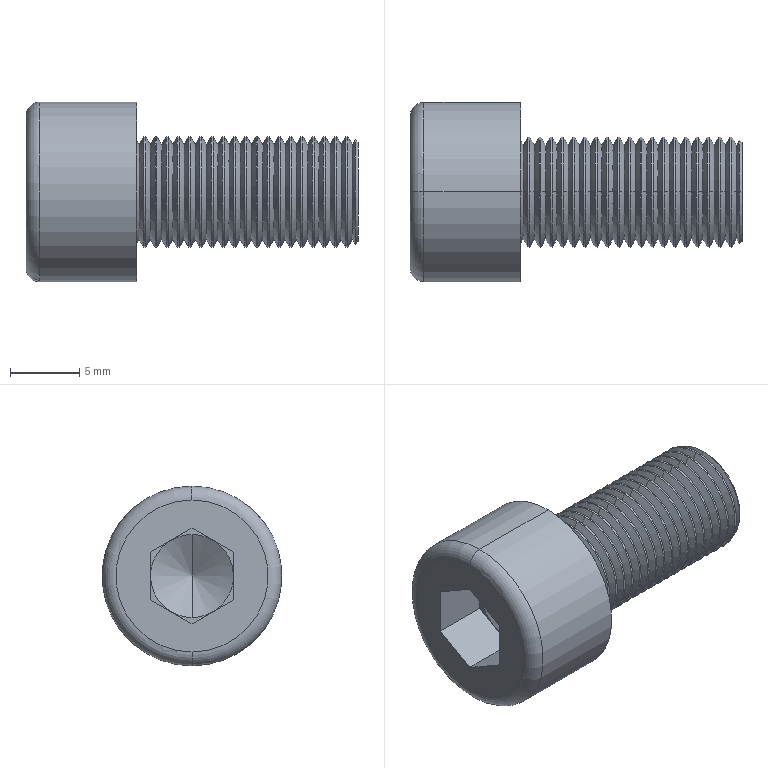Part | STEP file | PN_0008_Default<As Machined> | 1 solid | 144 faces | box 24 x 13 x 13 mm | volume 1618 mm3 | cone 84 | cylinder 42 | plane 16 | torus 2 | commonest cylinder face diameters 8 x38 9.353 x2 13 x2